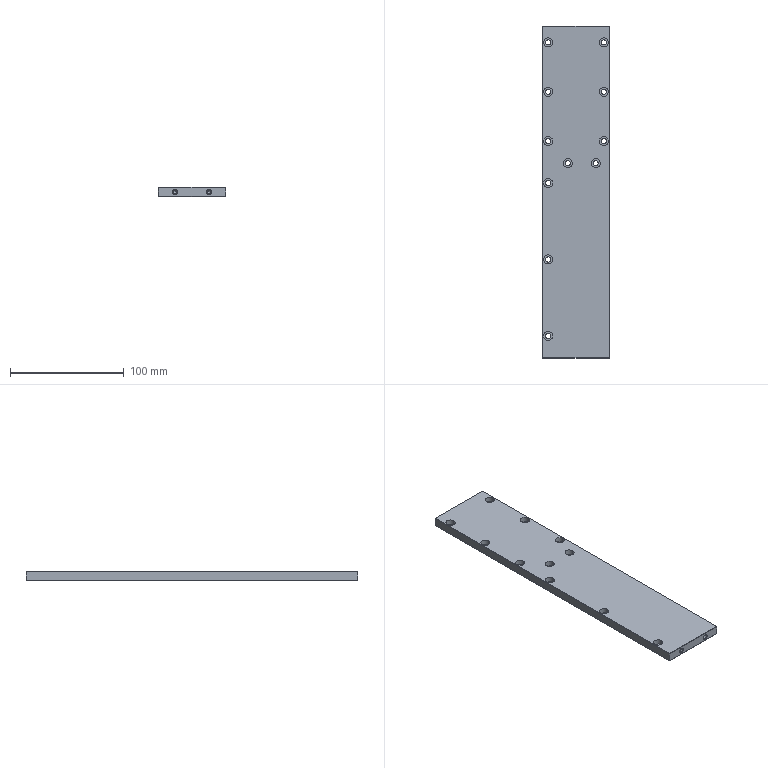Part | NX | 1 solid | 89 faces | box 59 x 291.5 x 8 mm | volume 134257 mm3 | cylinder 52 | plane 29 | cone 8 | commonest cylinder face diameters 4.5 x22 8 x22 3.3 x8